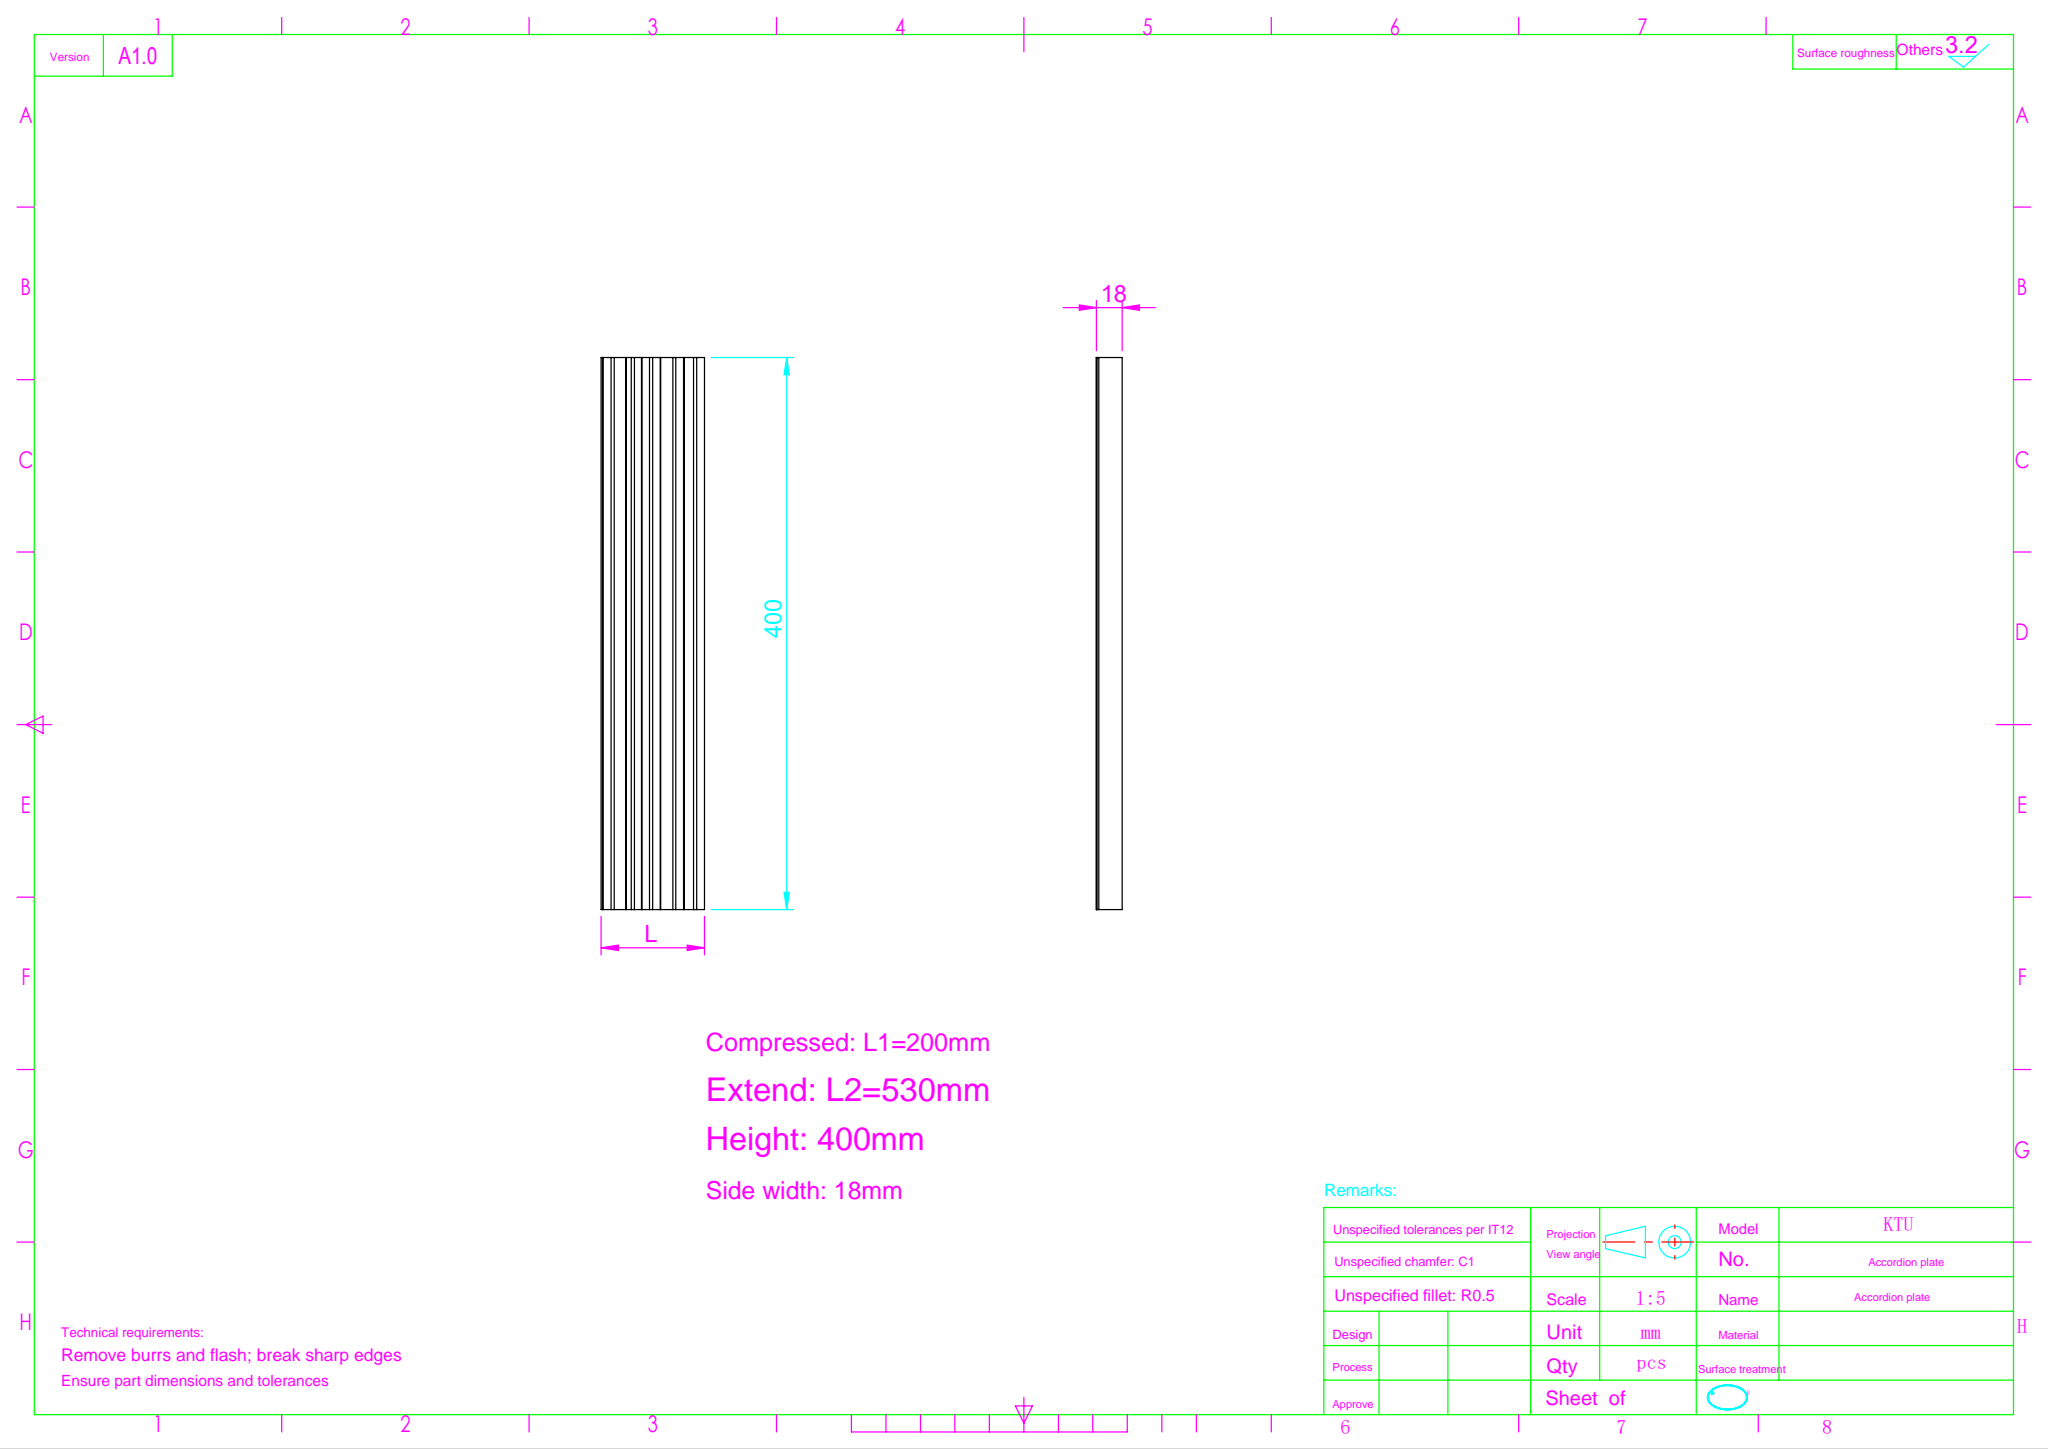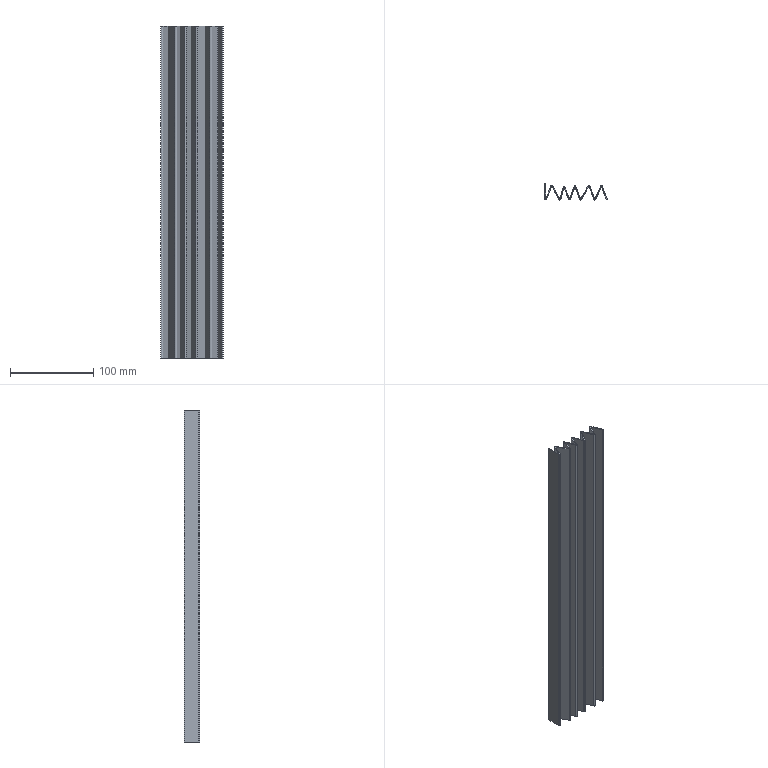Part | SolidWorks | features FlatPattern 1, SMBaseFlange 1, SheetMetal 1 | 1 solid | 86 faces | box 74.992 x 18.732 x 400 mm | volume 77618 mm3 | plane 66 | cylinder 20 | commonest cylinder face diameters 0.4 x10 2.4 x10